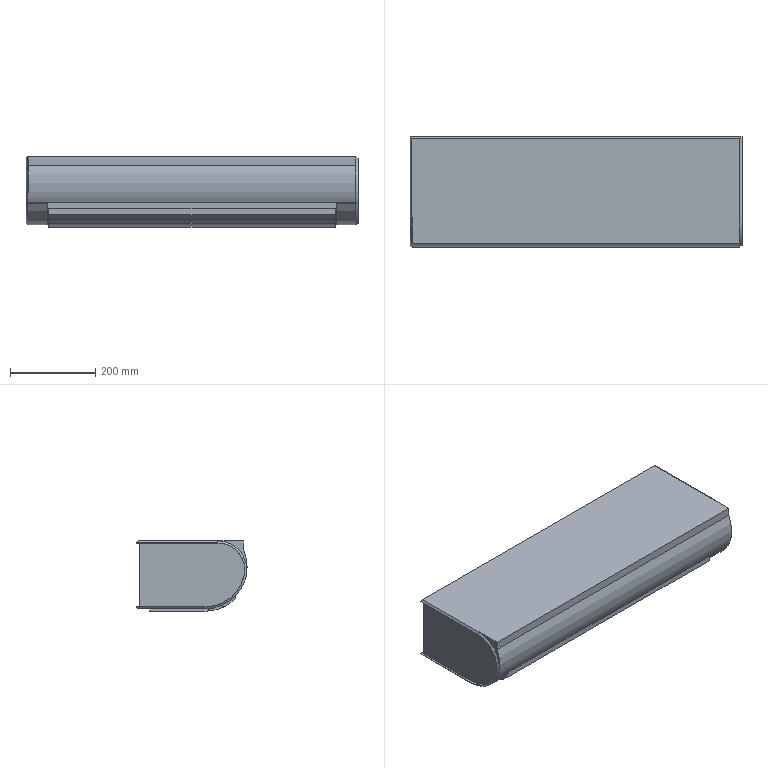Part | NX | features BREP 2 | 2 solids | 96 faces | box 780 x 258.929 x 165 mm | volume 11482720 mm3 | plane 61 | cylinder 27 | cone 4 | torus 4 | commonest cylinder face diameters 2 x4 10 x4 187.857 x4 8.115 x3 197.857 x3 207.857 x3